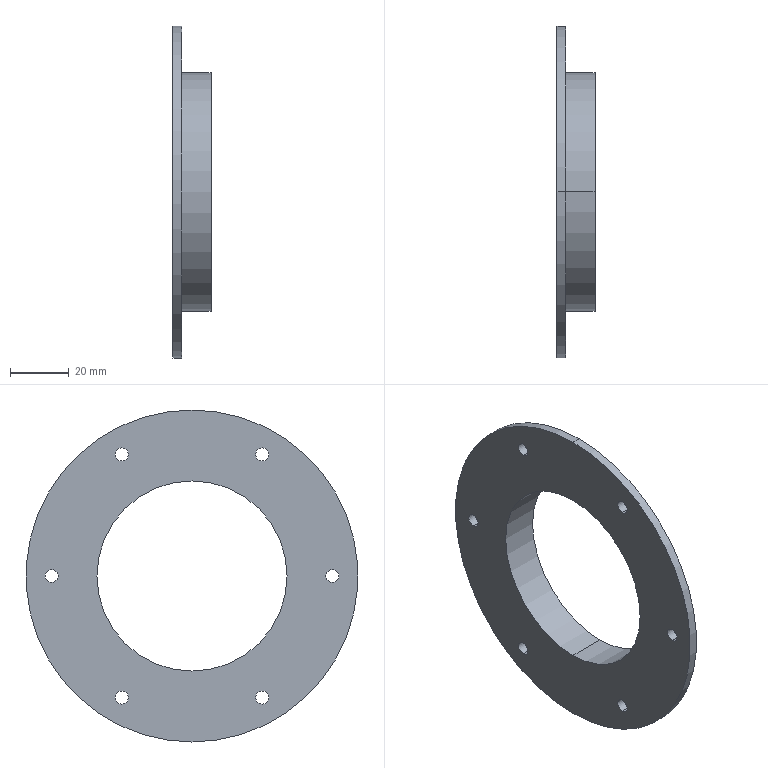Part | SolidWorks | features Chamfer 2, CirPattern 1, ICE 1, Revolution 1 | 1 solid | 31 faces | box 13 x 113.5 x 113.5 mm | volume 34508 mm3 | cylinder 22 | plane 5 | cone 4 | commonest cylinder face diameters 4.5 x12 65 x2 68.6 x2 71.5 x2 81.5 x2 113.5 x2
STEP:
#1=CARTESIAN_POINT('',(0.,24.,43.819));
#2=VERTEX_POINT('',#1);
#3=CARTESIAN_POINT('',(0.,24.,39.319));
#4=VERTEX_POINT('',#3);
#5=CARTESIAN_POINT('',(0.,24.,41.569));
#6=DIRECTION('',(1.,0.,0.));
#7=DIRECTION('',(0.,0.,-1.));
#8=AXIS2_PLACEMENT_3D('',#5,#6,#7);
#9=CIRCLE('',#8,2.25);
#10=EDGE_CURVE('',#2,#4,#9,.T.);
#11=ORIENTED_EDGE('',*,*,#10,.F.);
#12=CARTESIAN_POINT('',(3.,24.,43.819));
#13=VERTEX_POINT('',#12);
#14=CARTESIAN_POINT('',(-7.,24.,43.819));
#15=DIRECTION('',(1.,0.,0.));
#16=VECTOR('',#15,1000.);
#17=LINE('',#14,#16);
#18=EDGE_CURVE('',#2,#13,#17,.T.);
#19=ORIENTED_EDGE('',*,*,#18,.T.);
#20=CARTESIAN_POINT('',(3.,24.,39.319));
#21=VERTEX_POINT('',#20);
#22=CARTESIAN_POINT('',(3.,24.,41.569));
#23=DIRECTION('',(1.,0.,0.));
#24=DIRECTION('',(0.,0.866,-0.5));
#25=AXIS2_PLACEMENT_3D('',#22,#23,#24);
#26=CIRCLE('',#25,2.25);
#27=EDGE_CURVE('',#13,#21,#26,.T.);
#28=ORIENTED_EDGE('',*,*,#27,.T.);
#29=CARTESIAN_POINT('',(-7.,24.,39.319));
#30=DIRECTION('',(1.,0.,0.));
#31=VECTOR('',#30,1000.);
#32=LINE('',#29,#31);
#33=EDGE_CURVE('',#4,#21,#32,.T.);
#34=ORIENTED_EDGE('',*,*,#33,.F.);
#35=EDGE_LOOP('',(#11,#19,#28,#34));
#36=FACE_OUTER_BOUND('',#35,.T.);
#37=CARTESIAN_POINT('',(-7.,24.,41.569));
#38=DIRECTION('',(1.,0.,0.));
#39=DIRECTION('',(0.,0.,-1.));
#40=AXIS2_PLACEMENT_3D('',#37,#38,#39);
#41=CYLINDRICAL_SURFACE('',#40,2.25);
#42=ADVANCED_FACE('',(#36),#41,.F.);
#43=CARTESIAN_POINT('',(0.,-24.,43.819));
#44=VERTEX_POINT('',#43);
#45=CARTESIAN_POINT('',(0.,-24.,39.319));
#46=VERTEX_POINT('',#45);
#47=CARTESIAN_POINT('',(0.,-24.,41.569));
#48=DIRECTION('',(1.,0.,0.));
#49=DIRECTION('',(0.,0.,-1.));
#50=AXIS2_PLACEMENT_3D('',#47,#48,#49);
#51=CIRCLE('',#50,2.25);
#52=EDGE_CURVE('',#44,#46,#51,.T.);
#53=ORIENTED_EDGE('',*,*,#52,.F.);
#54=CARTESIAN_POINT('',(3.,-24.,43.819));
#55=VERTEX_POINT('',#54);
#56=CARTESIAN_POINT('',(-7.,-24.,43.819));
#57=DIRECTION('',(1.,0.,0.));
#58=VECTOR('',#57,1000.);
#59=LINE('',#56,#58);
#60=EDGE_CURVE('',#44,#55,#59,.T.);
#61=ORIENTED_EDGE('',*,*,#60,.T.);
#62=CARTESIAN_POINT('',(3.,-24.,39.319));
#63=VERTEX_POINT('',#62);
#64=CARTESIAN_POINT('',(3.,-24.,41.569));
#65=DIRECTION('',(1.,0.,0.));
#66=DIRECTION('',(0.,0.866,0.5));
#67=AXIS2_PLACEMENT_3D('',#64,#65,#66);
#68=CIRCLE('',#67,2.25);
#69=EDGE_CURVE('',#55,#63,#68,.T.);
#70=ORIENTED_EDGE('',*,*,#69,.T.);
#71=CARTESIAN_POINT('',(-7.,-24.,39.319));
#72=DIRECTION('',(1.,0.,0.));
#73=VECTOR('',#72,1000.);
#74=LINE('',#71,#73);
#75=EDGE_CURVE('',#46,#63,#74,.T.);
#76=ORIENTED_EDGE('',*,*,#75,.F.);
#77=EDGE_LOOP('',(#53,#61,#70,#76));
#78=FACE_OUTER_BOUND('',#77,.T.);
#79=CARTESIAN_POINT('',(-7.,-24.,41.569));
#80=DIRECTION('',(1.,0.,0.));
#81=DIRECTION('',(0.,0.,-1.));
#82=AXIS2_PLACEMENT_3D('',#79,#80,#81);
#83=CYLINDRICAL_SURFACE('',#82,2.25);
#84=ADVANCED_FACE('',(#78),#83,.F.);
#85=CARTESIAN_POINT('',(0.,-48.,2.25));
#86=VERTEX_POINT('',#85);
#87=CARTESIAN_POINT('',(0.,-48.,-2.25));
#88=VERTEX_POINT('',#87);
#89=CARTESIAN_POINT('',(0.,-48.,0.));
#90=DIRECTION('',(1.,0.,0.));
#91=DIRECTION('',(0.,0.,-1.));
#92=AXIS2_PLACEMENT_3D('',#89,#90,#91);
#93=CIRCLE('',#92,2.25);
#94=EDGE_CURVE('',#86,#88,#93,.T.);
#95=ORIENTED_EDGE('',*,*,#94,.F.);
#96=CARTESIAN_POINT('',(3.,-48.,2.25));
#97=VERTEX_POINT('',#96);
#98=CARTESIAN_POINT('',(-7.,-48.,2.25));
#99=DIRECTION('',(1.,0.,0.));
#100=VECTOR('',#99,1000.);
#101=LINE('',#98,#100);
#102=EDGE_CURVE('',#86,#97,#101,.T.);
#103=ORIENTED_EDGE('',*,*,#102,.T.);
#104=CARTESIAN_POINT('',(3.,-48.,-2.25));
#105=VERTEX_POINT('',#104);
#106=CARTESIAN_POINT('',(3.,-48.,0.));
#107=DIRECTION('',(1.,0.,0.));
#108=DIRECTION('',(0.,0.,1.));
#109=AXIS2_PLACEMENT_3D('',#106,#107,#108);
#110=CIRCLE('',#109,2.25);
#111=EDGE_CURVE('',#97,#105,#110,.T.);
#112=ORIENTED_EDGE('',*,*,#111,.T.);
#113=CARTESIAN_POINT('',(-7.,-48.,-2.25));
#114=DIRECTION('',(1.,0.,0.));
#115=VECTOR('',#114,1000.);
#116=LINE('',#113,#115);
#117=EDGE_CURVE('',#88,#105,#116,.T.);
#118=ORIENTED_EDGE('',*,*,#117,.F.);
#119=EDGE_LOOP('',(#95,#103,#112,#118));
#120=FACE_OUTER_BOUND('',#119,.T.);
#121=CARTESIAN_POINT('',(-7.,-48.,0.));
#122=DIRECTION('',(1.,0.,0.));
#123=DIRECTION('',(0.,0.,-1.));
#124=AXIS2_PLACEMENT_3D('',#121,#122,#123);
#125=CYLINDRICAL_SURFACE('',#124,2.25);
#126=ADVANCED_FACE('',(#120),#125,.F.);
#127=CARTESIAN_POINT('',(0.,-24.,-39.319));
#128=VERTEX_POINT('',#127);
#129=CARTESIAN_POINT('',(0.,-24.,-43.819));
#130=VERTEX_POINT('',#129);
#131=CARTESIAN_POINT('',(0.,-24.,-41.569));
#132=DIRECTION('',(1.,0.,0.));
#133=DIRECTION('',(0.,0.,-1.));
#134=AXIS2_PLACEMENT_3D('',#131,#132,#133);
#135=CIRCLE('',#134,2.25);
#136=EDGE_CURVE('',#128,#130,#135,.T.);
#137=ORIENTED_EDGE('',*,*,#136,.F.);
#138=CARTESIAN_POINT('',(3.,-24.,-39.319));
#139=VERTEX_POINT('',#138);
#140=CARTESIAN_POINT('',(-7.,-24.,-39.319));
#141=DIRECTION('',(1.,0.,0.));
#142=VECTOR('',#141,1000.);
#143=LINE('',#140,#142);
#144=EDGE_CURVE('',#128,#139,#143,.T.);
#145=ORIENTED_EDGE('',*,*,#144,.T.);
#146=CARTESIAN_POINT('',(3.,-24.,-43.819));
#147=VERTEX_POINT('',#146);
#148=CARTESIAN_POINT('',(3.,-24.,-41.569));
#149=DIRECTION('',(1.,0.,0.));
#150=DIRECTION('',(0.,-0.866,0.5));
#151=AXIS2_PLACEMENT_3D('',#148,#149,#150);
#152=CIRCLE('',#151,2.25);
#153=EDGE_CURVE('',#139,#147,#152,.T.);
#154=ORIENTED_EDGE('',*,*,#153,.T.);
#155=CARTESIAN_POINT('',(-7.,-24.,-43.819));
#156=DIRECTION('',(1.,0.,0.));
#157=VECTOR('',#156,1000.);
#158=LINE('',#155,#157);
#159=EDGE_CURVE('',#130,#147,#158,.T.);
#160=ORIENTED_EDGE('',*,*,#159,.F.);
#161=EDGE_LOOP('',(#137,#145,#154,#160));
#162=FACE_OUTER_BOUND('',#161,.T.);
#163=CARTESIAN_POINT('',(-7.,-24.,-41.569));
#164=DIRECTION('',(1.,0.,0.));
#165=DIRECTION('',(0.,0.,-1.));
#166=AXIS2_PLACEMENT_3D('',#163,#164,#165);
#167=CYLINDRICAL_SURFACE('',#166,2.25);
#168=ADVANCED_FACE('',(#162),#167,.F.);
#169=CARTESIAN_POINT('',(0.,24.,-39.319));
#170=VERTEX_POINT('',#169);
#171=CARTESIAN_POINT('',(0.,24.,-43.819));
#172=VERTEX_POINT('',#171);
#173=CARTESIAN_POINT('',(0.,24.,-41.569));
#174=DIRECTION('',(1.,0.,0.));
#175=DIRECTION('',(0.,0.,-1.));
#176=AXIS2_PLACEMENT_3D('',#173,#174,#175);
#177=CIRCLE('',#176,2.25);
#178=EDGE_CURVE('',#170,#172,#177,.T.);
#179=ORIENTED_EDGE('',*,*,#178,.F.);
#180=CARTESIAN_POINT('',(3.,24.,-39.319));
#181=VERTEX_POINT('',#180);
#182=CARTESIAN_POINT('',(-7.,24.,-39.319));
#183=DIRECTION('',(1.,0.,0.));
#184=VECTOR('',#183,1000.);
#185=LINE('',#182,#184);
#186=EDGE_CURVE('',#170,#181,#185,.T.);
#187=ORIENTED_EDGE('',*,*,#186,.T.);
#188=CARTESIAN_POINT('',(3.,24.,-43.819));
#189=VERTEX_POINT('',#188);
#190=CARTESIAN_POINT('',(3.,24.,-41.569));
#191=DIRECTION('',(1.,0.,0.));
#192=DIRECTION('',(0.,-0.866,-0.5));
#193=AXIS2_PLACEMENT_3D('',#190,#191,#192);
#194=CIRCLE('',#193,2.25);
#195=EDGE_CURVE('',#181,#189,#194,.T.);
#196=ORIENTED_EDGE('',*,*,#195,.T.);
#197=CARTESIAN_POINT('',(-7.,24.,-43.819));
#198=DIRECTION('',(1.,0.,0.));
#199=VECTOR('',#198,1000.);
#200=LINE('',#197,#199);
#201=EDGE_CURVE('',#172,#189,#200,.T.);
#202=ORIENTED_EDGE('',*,*,#201,.F.);
#203=EDGE_LOOP('',(#179,#187,#196,#202));
#204=FACE_OUTER_BOUND('',#203,.T.);
#205=CARTESIAN_POINT('',(-7.,24.,-41.569));
#206=DIRECTION('',(1.,0.,0.));
#207=DIRECTION('',(0.,0.,-1.));
#208=AXIS2_PLACEMENT_3D('',#205,#206,#207);
#209=CYLINDRICAL_SURFACE('',#208,2.25);
#210=ADVANCED_FACE('',(#204),#209,.F.);
#211=CARTESIAN_POINT('',(0.,48.,2.25));
#212=VERTEX_POINT('',#211);
#213=CARTESIAN_POINT('',(0.,48.,-2.25));
#214=VERTEX_POINT('',#213);
#215=CARTESIAN_POINT('',(0.,48.,0.));
#216=DIRECTION('',(1.,0.,0.));
#217=DIRECTION('',(0.,0.,-1.));
#218=AXIS2_PLACEMENT_3D('',#215,#216,#217);
#219=CIRCLE('',#218,2.25);
#220=EDGE_CURVE('',#212,#214,#219,.T.);
#221=ORIENTED_EDGE('',*,*,#220,.F.);
#222=CARTESIAN_POINT('',(3.,48.,2.25));
#223=VERTEX_POINT('',#222);
#224=CARTESIAN_POINT('',(-7.,48.,2.25));
#225=DIRECTION('',(1.,0.,0.));
#226=VECTOR('',#225,1000.);
#227=LINE('',#224,#226);
#228=EDGE_CURVE('',#212,#223,#227,.T.);
#229=ORIENTED_EDGE('',*,*,#228,.T.);
#230=CARTESIAN_POINT('',(3.,48.,-2.25));
#231=VERTEX_POINT('',#230);
#232=CARTESIAN_POINT('',(3.,48.,0.));
#233=DIRECTION('',(1.,0.,0.));
#234=DIRECTION('',(0.,0.,-1.));
#235=AXIS2_PLACEMENT_3D('',#232,#233,#234);
#236=CIRCLE('',#235,2.25);
#237=EDGE_CURVE('',#223,#231,#236,.T.);
#238=ORIENTED_EDGE('',*,*,#237,.T.);
#239=CARTESIAN_POINT('',(-7.,48.,-2.25));
#240=DIRECTION('',(1.,0.,0.));
#241=VECTOR('',#240,1000.);
#242=LINE('',#239,#241);
#243=EDGE_CURVE('',#214,#231,#242,.T.);
#244=ORIENTED_EDGE('',*,*,#243,.F.);
#245=EDGE_LOOP('',(#221,#229,#238,#244));
#246=FACE_OUTER_BOUND('',#245,.T.);
#247=CARTESIAN_POINT('',(-7.,48.,0.));
#248=DIRECTION('',(1.,0.,0.));
#249=DIRECTION('',(0.,0.,-1.));
#250=AXIS2_PLACEMENT_3D('',#247,#248,#249);
#251=CYLINDRICAL_SURFACE('',#250,2.25);
#252=ADVANCED_FACE('',(#246),#251,.F.);
#253=CARTESIAN_POINT('',(13.,0.,-33.3));
#254=VERTEX_POINT('',#253);
#255=CARTESIAN_POINT('',(13.,0.,33.3));
#256=VERTEX_POINT('',#255);
#257=CARTESIAN_POINT('',(13.,0.,0.));
#258=DIRECTION('',(1.,0.,0.));
#259=DIRECTION('',(0.,0.,1.));
#260=AXIS2_PLACEMENT_3D('',#257,#258,#259);
#261=CIRCLE('',#260,33.3);
#262=EDGE_CURVE('',#254,#256,#261,.T.);
#263=ORIENTED_EDGE('',*,*,#262,.F.);
#264=CARTESIAN_POINT('',(12.,0.,-34.3));
#265=VERTEX_POINT('',#264);
#266=CARTESIAN_POINT('',(12.,0.,-34.3));
#267=DIRECTION('',(-0.7071,0.,-0.7071));
#268=VECTOR('',#267,1000.);
#269=LINE('',#266,#268);
#270=EDGE_CURVE('',#254,#265,#269,.T.);
#271=ORIENTED_EDGE('',*,*,#270,.T.);
#272=CARTESIAN_POINT('',(12.,0.,34.3));
#273=VERTEX_POINT('',#272);
#274=CARTESIAN_POINT('',(12.,0.,0.));
#275=DIRECTION('',(-1.,0.,0.));
#276=DIRECTION('',(0.,0.,1.));
#277=AXIS2_PLACEMENT_3D('',#274,#275,#276);
#278=CIRCLE('',#277,34.3);
#279=EDGE_CURVE('',#273,#265,#278,.T.);
#280=ORIENTED_EDGE('',*,*,#279,.F.);
#281=CARTESIAN_POINT('',(12.,0.,34.3));
#282=DIRECTION('',(-0.7071,0.,0.7071));
#283=VECTOR('',#282,1000.);
#284=LINE('',#281,#283);
#285=EDGE_CURVE('',#256,#273,#284,.T.);
#286=ORIENTED_EDGE('',*,*,#285,.F.);
#287=EDGE_LOOP('',(#263,#271,#280,#286));
#288=FACE_OUTER_BOUND('',#287,.T.);
#289=CARTESIAN_POINT('',(12.,0.,0.));
#290=DIRECTION('',(-1.,0.,0.));
#291=DIRECTION('',(0.,0.,1.));
#292=AXIS2_PLACEMENT_3D('',#289,#290,#291);
#293=CONICAL_SURFACE('',#292,34.3,0.7854);
#294=ADVANCED_FACE('',(#288),#293,.T.);
#295=CARTESIAN_POINT('',(9.,0.,35.75));
#296=VERTEX_POINT('',#295);
#297=CARTESIAN_POINT('',(9.,0.,-35.75));
#298=VERTEX_POINT('',#297);
#299=CARTESIAN_POINT('',(9.,0.,0.));
#300=DIRECTION('',(1.,0.,0.));
#301=DIRECTION('',(0.,0.,1.));
#302=AXIS2_PLACEMENT_3D('',#299,#300,#301);
#303=CIRCLE('',#302,35.75);
#304=EDGE_CURVE('',#296,#298,#303,.T.);
#305=ORIENTED_EDGE('',*,*,#304,.F.);
#306=CARTESIAN_POINT('',(13.,0.,38.551));
#307=VERTEX_POINT('',#306);
#308=CARTESIAN_POINT('',(13.,0.,38.551));
#309=DIRECTION('',(0.8192,0.,0.5736));
#310=VECTOR('',#309,1000.);
#311=LINE('',#308,#310);
#312=EDGE_CURVE('',#296,#307,#311,.T.);
#313=ORIENTED_EDGE('',*,*,#312,.T.);
#314=CARTESIAN_POINT('',(13.,0.,-38.551));
#315=VERTEX_POINT('',#314);
#316=CARTESIAN_POINT('',(13.,0.,0.));
#317=DIRECTION('',(-1.,0.,0.));
#318=DIRECTION('',(0.,0.,1.));
#319=AXIS2_PLACEMENT_3D('',#316,#317,#318);
#320=CIRCLE('',#319,38.551);
#321=EDGE_CURVE('',#315,#307,#320,.T.);
#322=ORIENTED_EDGE('',*,*,#321,.F.);
#323=CARTESIAN_POINT('',(13.,0.,-38.551));
#324=DIRECTION('',(0.8192,0.,-0.5736));
#325=VECTOR('',#324,1000.);
#326=LINE('',#323,#325);
#327=EDGE_CURVE('',#298,#315,#326,.T.);
#328=ORIENTED_EDGE('',*,*,#327,.F.);
#329=EDGE_LOOP('',(#305,#313,#322,#328));
#330=FACE_OUTER_BOUND('',#329,.T.);
#331=CARTESIAN_POINT('',(13.,0.,0.));
#332=DIRECTION('',(1.,0.,0.));
#333=DIRECTION('',(0.,0.,-1.));
#334=AXIS2_PLACEMENT_3D('',#331,#332,#333);
#335=CONICAL_SURFACE('',#334,38.551,0.6109);
#336=ADVANCED_FACE('',(#330),#335,.F.);
#337=CARTESIAN_POINT('',(3.,0.,56.75));
#338=VERTEX_POINT('',#337);
#339=CARTESIAN_POINT('',(3.,0.,-56.75));
#340=VERTEX_POINT('',#339);
#341=CARTESIAN_POINT('',(3.,0.,0.));
#342=DIRECTION('',(-1.,0.,0.));
#343=DIRECTION('',(0.,0.,1.));
#344=AXIS2_PLACEMENT_3D('',#341,#342,#343);
#345=CIRCLE('',#344,56.75);
#346=EDGE_CURVE('',#338,#340,#345,.T.);
#347=ORIENTED_EDGE('',*,*,#346,.T.);
#348=CARTESIAN_POINT('',(0.,0.,-56.75));
#349=VERTEX_POINT('',#348);
#350=CARTESIAN_POINT('',(0.,0.,-56.75));
#351=DIRECTION('',(-1.,0.,0.));
#352=VECTOR('',#351,1000.);
#353=LINE('',#350,#352);
#354=EDGE_CURVE('',#340,#349,#353,.T.);
#355=ORIENTED_EDGE('',*,*,#354,.T.);
#356=CARTESIAN_POINT('',(0.,0.,56.75));
#357=VERTEX_POINT('',#356);
#358=CARTESIAN_POINT('',(0.,0.,0.));
#359=DIRECTION('',(-1.,0.,0.));
#360=DIRECTION('',(0.,0.,1.));
#361=AXIS2_PLACEMENT_3D('',#358,#359,#360);
#362=CIRCLE('',#361,56.75);
#363=EDGE_CURVE('',#357,#349,#362,.T.);
#364=ORIENTED_EDGE('',*,*,#363,.F.);
#365=CARTESIAN_POINT('',(0.,0.,56.75));
#366=DIRECTION('',(-1.,0.,0.));
#367=VECTOR('',#366,1000.);
#368=LINE('',#365,#367);
#369=EDGE_CURVE('',#338,#357,#368,.T.);
#370=ORIENTED_EDGE('',*,*,#369,.F.);
#371=EDGE_LOOP('',(#347,#355,#364,#370));
#372=FACE_OUTER_BOUND('',#371,.T.);
#373=CARTESIAN_POINT('',(0.,0.,0.));
#374=DIRECTION('',(-1.,0.,0.));
#375=DIRECTION('',(0.,0.,1.));
#376=AXIS2_PLACEMENT_3D('',#373,#374,#375);
#377=CYLINDRICAL_SURFACE('',#376,56.75);
#378=ADVANCED_FACE('',(#372),#377,.T.);
#379=CARTESIAN_POINT('',(13.,0.,40.75));
#380=VERTEX_POINT('',#379);
#381=CARTESIAN_POINT('',(13.,0.,-40.75));
#382=VERTEX_POINT('',#381);
#383=CARTESIAN_POINT('',(13.,0.,0.));
#384=DIRECTION('',(-1.,0.,0.));
#385=DIRECTION('',(0.,0.,1.));
#386=AXIS2_PLACEMENT_3D('',#383,#384,#385);
#387=CIRCLE('',#386,40.75);
#388=EDGE_CURVE('',#380,#382,#387,.T.);
#389=ORIENTED_EDGE('',*,*,#388,.T.);
#390=CARTESIAN_POINT('',(3.,0.,-40.75));
#391=VERTEX_POINT('',#390);
#392=CARTESIAN_POINT('',(0.,0.,-40.75));
#393=DIRECTION('',(-1.,0.,0.));
#394=VECTOR('',#393,1000.);
#395=LINE('',#392,#394);
#396=EDGE_CURVE('',#382,#391,#395,.T.);
#397=ORIENTED_EDGE('',*,*,#396,.T.);
#398=CARTESIAN_POINT('',(3.,0.,40.75));
#399=VERTEX_POINT('',#398);
#400=CARTESIAN_POINT('',(3.,0.,0.));
#401=DIRECTION('',(-1.,0.,0.));
#402=DIRECTION('',(0.,0.,1.));
#403=AXIS2_PLACEMENT_3D('',#400,#401,#402);
#404=CIRCLE('',#403,40.75);
#405=EDGE_CURVE('',#399,#391,#404,.T.);
#406=ORIENTED_EDGE('',*,*,#405,.F.);
#407=CARTESIAN_POINT('',(0.,0.,40.75));
#408=DIRECTION('',(-1.,0.,0.));
#409=VECTOR('',#408,1000.);
#410=LINE('',#407,#409);
#411=EDGE_CURVE('',#380,#399,#410,.T.);
#412=ORIENTED_EDGE('',*,*,#411,.F.);
#413=EDGE_LOOP('',(#389,#397,#406,#412));
#414=FACE_OUTER_BOUND('',#413,.T.);
#415=CARTESIAN_POINT('',(0.,0.,0.));
#416=DIRECTION('',(-1.,0.,0.));
#417=DIRECTION('',(0.,0.,1.));
#418=AXIS2_PLACEMENT_3D('',#415,#416,#417);
#419=CYLINDRICAL_SURFACE('',#418,40.75);
#420=ADVANCED_FACE('',(#414),#419,.T.);
#421=ORIENTED_EDGE('',*,*,#304,.T.);
#422=CARTESIAN_POINT('',(3.,0.,-35.75));
#423=VERTEX_POINT('',#422);
#424=CARTESIAN_POINT('',(0.,0.,-35.75));
#425=DIRECTION('',(-1.,0.,0.));
#426=VECTOR('',#425,1000.);
#427=LINE('',#424,#426);
#428=EDGE_CURVE('',#298,#423,#427,.T.);
#429=ORIENTED_EDGE('',*,*,#428,.T.);
#430=CARTESIAN_POINT('',(3.,0.,35.75));
#431=VERTEX_POINT('',#430);
#432=CARTESIAN_POINT('',(3.,0.,0.));
#433=DIRECTION('',(-1.,0.,0.));
#434=DIRECTION('',(0.,0.,1.));
#435=AXIS2_PLACEMENT_3D('',#432,#433,#434);
#436=CIRCLE('',#435,35.75);
#437=EDGE_CURVE('',#423,#431,#436,.T.);
#438=ORIENTED_EDGE('',*,*,#437,.T.);
#439=CARTESIAN_POINT('',(0.,0.,35.75));
#440=DIRECTION('',(-1.,0.,0.));
#441=VECTOR('',#440,1000.);
#442=LINE('',#439,#441);
#443=EDGE_CURVE('',#296,#431,#442,.T.);
#444=ORIENTED_EDGE('',*,*,#443,.F.);
#445=EDGE_LOOP('',(#421,#429,#438,#444));
#446=FACE_OUTER_BOUND('',#445,.T.);
#447=CARTESIAN_POINT('',(0.,0.,0.));
#448=DIRECTION('',(-1.,0.,0.));
#449=DIRECTION('',(0.,0.,1.));
#450=AXIS2_PLACEMENT_3D('',#447,#448,#449);
#451=CYLINDRICAL_SURFACE('',#450,35.75);
#452=ADVANCED_FACE('',(#446),#451,.F.);
#453=ORIENTED_EDGE('',*,*,#279,.T.);
#454=CARTESIAN_POINT('',(3.,0.,-34.3));
#455=VERTEX_POINT('',#454);
#456=CARTESIAN_POINT('',(0.,0.,-34.3));
#457=DIRECTION('',(-1.,0.,0.));
#458=VECTOR('',#457,1000.);
#459=LINE('',#456,#458);
#460=EDGE_CURVE('',#265,#455,#459,.T.);
#461=ORIENTED_EDGE('',*,*,#460,.T.);
#462=CARTESIAN_POINT('',(3.,0.,34.3));
#463=VERTEX_POINT('',#462);
#464=CARTESIAN_POINT('',(3.,0.,0.));
#465=DIRECTION('',(-1.,0.,0.));
#466=DIRECTION('',(0.,0.,1.));
#467=AXIS2_PLACEMENT_3D('',#464,#465,#466);
#468=CIRCLE('',#467,34.3);
#469=EDGE_CURVE('',#463,#455,#468,.T.);
#470=ORIENTED_EDGE('',*,*,#469,.F.);
#471=CARTESIAN_POINT('',(0.,0.,34.3));
#472=DIRECTION('',(-1.,0.,0.));
#473=VECTOR('',#472,1000.);
#474=LINE('',#471,#473);
#475=EDGE_CURVE('',#273,#463,#474,.T.);
#476=ORIENTED_EDGE('',*,*,#475,.F.);
#477=EDGE_LOOP('',(#453,#461,#470,#476));
#478=FACE_OUTER_BOUND('',#477,.T.);
#479=CARTESIAN_POINT('',(0.,0.,0.));
#480=DIRECTION('',(-1.,0.,0.));
#481=DIRECTION('',(0.,0.,1.));
#482=AXIS2_PLACEMENT_3D('',#479,#480,#481);
#483=CYLINDRICAL_SURFACE('',#482,34.3);
#484=ADVANCED_FACE('',(#478),#483,.T.);
#485=CARTESIAN_POINT('',(13.,0.,-32.5));
#486=VERTEX_POINT('',#485);
#487=CARTESIAN_POINT('',(13.,0.,32.5));
#488=VERTEX_POINT('',#487);
#489=CARTESIAN_POINT('',(13.,0.,0.));
#490=DIRECTION('',(-1.,0.,0.));
#491=DIRECTION('',(0.,0.,1.));
#492=AXIS2_PLACEMENT_3D('',#489,#490,#491);
#493=CIRCLE('',#492,32.5);
#494=EDGE_CURVE('',#486,#488,#493,.T.);
#495=ORIENTED_EDGE('',*,*,#494,.F.);
#496=CARTESIAN_POINT('',(0.,0.,-32.5));
#497=VERTEX_POINT('',#496);
#498=CARTESIAN_POINT('',(0.,0.,-32.5));
#499=DIRECTION('',(-1.,0.,0.));
#500=VECTOR('',#499,1000.);
#501=LINE('',#498,#500);
#502=EDGE_CURVE('',#486,#497,#501,.T.);
#503=ORIENTED_EDGE('',*,*,#502,.T.);
#504=CARTESIAN_POINT('',(0.,0.,32.5));
#505=VERTEX_POINT('',#504);
#506=CARTESIAN_POINT('',(0.,0.,0.));
#507=DIRECTION('',(-1.,0.,0.));
#508=DIRECTION('',(0.,0.,1.));
#509=AXIS2_PLACEMENT_3D('',#506,#507,#508);
#510=CIRCLE('',#509,32.5);
#511=EDGE_CURVE('',#497,#505,#510,.T.);
#512=ORIENTED_EDGE('',*,*,#511,.T.);
#513=CARTESIAN_POINT('',(0.,0.,32.5));
#514=DIRECTION('',(-1.,0.,0.));
#515=VECTOR('',#514,1000.);
#516=LINE('',#513,#515);
#517=EDGE_CURVE('',#488,#505,#516,.T.);
#518=ORIENTED_EDGE('',*,*,#517,.F.);
#519=EDGE_LOOP('',(#495,#503,#512,#518));
#520=FACE_OUTER_BOUND('',#519,.T.);
#521=CARTESIAN_POINT('',(0.,0.,0.));
#522=DIRECTION('',(-1.,0.,0.));
#523=DIRECTION('',(0.,0.,1.));
#524=AXIS2_PLACEMENT_3D('',#521,#522,#523);
#525=CYLINDRICAL_SURFACE('',#524,32.5);
#526=ADVANCED_FACE('',(#520),#525,.F.);
#527=CARTESIAN_POINT('',(0.,24.,41.569));
#528=DIRECTION('',(1.,0.,0.));
#529=DIRECTION('',(0.,0.,-1.));
#530=AXIS2_PLACEMENT_3D('',#527,#528,#529);
#531=CIRCLE('',#530,2.25);
#532=EDGE_CURVE('',#4,#2,#531,.T.);
#533=ORIENTED_EDGE('',*,*,#532,.T.);
#534=ORIENTED_EDGE('',*,*,#10,.T.);
#535=EDGE_LOOP('',(#533,#534));
#536=FACE_BOUND('',#535,.T.);
#537=CARTESIAN_POINT('',(0.,-24.,41.569));
#538=DIRECTION('',(1.,0.,0.));
#539=DIRECTION('',(0.,0.,-1.));
#540=AXIS2_PLACEMENT_3D('',#537,#538,#539);
#541=CIRCLE('',#540,2.25);
#542=EDGE_CURVE('',#46,#44,#541,.T.);
#543=ORIENTED_EDGE('',*,*,#542,.T.);
#544=ORIENTED_EDGE('',*,*,#52,.T.);
#545=EDGE_LOOP('',(#543,#544));
#546=FACE_BOUND('',#545,.T.);
#547=CARTESIAN_POINT('',(0.,-48.,0.));
#548=DIRECTION('',(1.,0.,0.));
#549=DIRECTION('',(0.,0.,-1.));
#550=AXIS2_PLACEMENT_3D('',#547,#548,#549);
#551=CIRCLE('',#550,2.25);
#552=EDGE_CURVE('',#88,#86,#551,.T.);
#553=ORIENTED_EDGE('',*,*,#552,.T.);
#554=ORIENTED_EDGE('',*,*,#94,.T.);
#555=EDGE_LOOP('',(#553,#554));
#556=FACE_BOUND('',#555,.T.);
#557=CARTESIAN_POINT('',(0.,-24.,-41.569));
#558=DIRECTION('',(1.,0.,0.));
#559=DIRECTION('',(0.,0.,-1.));
#560=AXIS2_PLACEMENT_3D('',#557,#558,#559);
#561=CIRCLE('',#560,2.25);
#562=EDGE_CURVE('',#130,#128,#561,.T.);
#563=ORIENTED_EDGE('',*,*,#562,.T.);
#564=ORIENTED_EDGE('',*,*,#136,.T.);
#565=EDGE_LOOP('',(#563,#564));
#566=FACE_BOUND('',#565,.T.);
#567=CARTESIAN_POINT('',(0.,24.,-41.569));
#568=DIRECTION('',(1.,0.,0.));
#569=DIRECTION('',(0.,0.,-1.));
#570=AXIS2_PLACEMENT_3D('',#567,#568,#569);
#571=CIRCLE('',#570,2.25);
#572=EDGE_CURVE('',#172,#170,#571,.T.);
#573=ORIENTED_EDGE('',*,*,#572,.T.);
#574=ORIENTED_EDGE('',*,*,#178,.T.);
#575=EDGE_LOOP('',(#573,#574));
#576=FACE_BOUND('',#575,.T.);
#577=CARTESIAN_POINT('',(0.,48.,0.));
#578=DIRECTION('',(1.,0.,0.));
#579=DIRECTION('',(0.,0.,-1.));
#580=AXIS2_PLACEMENT_3D('',#577,#578,#579);
#581=CIRCLE('',#580,2.25);
#582=EDGE_CURVE('',#214,#212,#581,.T.);
#583=ORIENTED_EDGE('',*,*,#582,.T.);
#584=ORIENTED_EDGE('',*,*,#220,.T.);
#585=EDGE_LOOP('',(#583,#584));
#586=FACE_BOUND('',#585,.T.);
#587=CARTESIAN_POINT('',(0.,0.,0.));
#588=DIRECTION('',(-1.,0.,0.));
#589=DIRECTION('',(0.,0.,1.));
#590=AXIS2_PLACEMENT_3D('',#587,#588,#589);
#591=CIRCLE('',#590,32.5);
#592=EDGE_CURVE('',#505,#497,#591,.T.);
#593=ORIENTED_EDGE('',*,*,#592,.F.);
#594=ORIENTED_EDGE('',*,*,#511,.F.);
#595=EDGE_LOOP('',(#593,#594));
#596=FACE_BOUND('',#595,.T.);
#597=ORIENTED_EDGE('',*,*,#363,.T.);
#598=CARTESIAN_POINT('',(0.,0.,0.));
#599=DIRECTION('',(-1.,0.,0.));
#600=DIRECTION('',(0.,0.,1.));
#601=AXIS2_PLACEMENT_3D('',#598,#599,#600);
#602=CIRCLE('',#601,56.75);
#603=EDGE_CURVE('',#349,#357,#602,.T.);
#604=ORIENTED_EDGE('',*,*,#603,.T.);
#605=EDGE_LOOP('',(#597,#604));
#606=FACE_OUTER_BOUND('',#605,.T.);
#607=CARTESIAN_POINT('',(0.,56.75,0.));
#608=DIRECTION('',(1.,0.,0.));
#609=DIRECTION('',(0.,0.,-1.));
#610=AXIS2_PLACEMENT_3D('',#607,#608,#609);
#611=PLANE('',#610);
#612=ADVANCED_FACE('',(#536,#546,#556,#566,#576,#586,#596,#606),#611,.F.);
#613=ORIENTED_EDGE('',*,*,#502,.F.);
#614=CARTESIAN_POINT('',(13.,0.,0.));
#615=DIRECTION('',(-1.,0.,0.));
#616=DIRECTION('',(0.,0.,1.));
#617=AXIS2_PLACEMENT_3D('',#614,#615,#616);
#618=CIRCLE('',#617,32.5);
#619=EDGE_CURVE('',#488,#486,#618,.T.);
#620=ORIENTED_EDGE('',*,*,#619,.F.);
#621=ORIENTED_EDGE('',*,*,#517,.T.);
#622=ORIENTED_EDGE('',*,*,#592,.T.);
#623=EDGE_LOOP('',(#613,#620,#621,#622));
#624=FACE_OUTER_BOUND('',#623,.T.);
#625=CARTESIAN_POINT('',(0.,0.,0.));
#626=DIRECTION('',(-1.,0.,0.));
#627=DIRECTION('',(0.,0.,1.));
#628=AXIS2_PLACEMENT_3D('',#625,#626,#627);
#629=CYLINDRICAL_SURFACE('',#628,32.5);
#630=ADVANCED_FACE('',(#624),#629,.F.);
#631=CARTESIAN_POINT('',(13.,0.,0.));
#632=DIRECTION('',(1.,0.,0.));
#633=DIRECTION('',(0.,0.,1.));
#634=AXIS2_PLACEMENT_3D('',#631,#632,#633);
#635=CIRCLE('',#634,33.3);
#636=EDGE_CURVE('',#256,#254,#635,.T.);
#637=ORIENTED_EDGE('',*,*,#636,.T.);
#638=ORIENTED_EDGE('',*,*,#262,.T.);
#639=EDGE_LOOP('',(#637,#638));
#640=FACE_OUTER_BOUND('',#639,.T.);
#641=ORIENTED_EDGE('',*,*,#619,.T.);
#642=ORIENTED_EDGE('',*,*,#494,.T.);
#643=EDGE_LOOP('',(#641,#642));
#644=FACE_BOUND('',#643,.T.);
#645=CARTESIAN_POINT('',(13.,32.5,0.));
#646=DIRECTION('',(-1.,0.,0.));
#647=DIRECTION('',(0.,0.,1.));
#648=AXIS2_PLACEMENT_3D('',#645,#646,#647);
#649=PLANE('',#648);
#650=ADVANCED_FACE('',(#640,#644),#649,.F.);
#651=ORIENTED_EDGE('',*,*,#460,.F.);
#652=CARTESIAN_POINT('',(12.,0.,0.));
#653=DIRECTION('',(-1.,0.,0.));
#654=DIRECTION('',(0.,0.,1.));
#655=AXIS2_PLACEMENT_3D('',#652,#653,#654);
#656=CIRCLE('',#655,34.3);
#657=EDGE_CURVE('',#265,#273,#656,.T.);
#658=ORIENTED_EDGE('',*,*,#657,.T.);
#659=ORIENTED_EDGE('',*,*,#475,.T.);
#660=CARTESIAN_POINT('',(3.,0.,0.));
#661=DIRECTION('',(-1.,0.,0.));
#662=DIRECTION('',(0.,0.,1.));
#663=AXIS2_PLACEMENT_3D('',#660,#661,#662);
#664=CIRCLE('',#663,34.3);
#665=EDGE_CURVE('',#455,#463,#664,.T.);
#666=ORIENTED_EDGE('',*,*,#665,.F.);
#667=EDGE_LOOP('',(#651,#658,#659,#666));
#668=FACE_OUTER_BOUND('',#667,.T.);
#669=CARTESIAN_POINT('',(0.,0.,0.));
#670=DIRECTION('',(-1.,0.,0.));
#671=DIRECTION('',(0.,0.,1.));
#672=AXIS2_PLACEMENT_3D('',#669,#670,#671);
#673=CYLINDRICAL_SURFACE('',#672,34.3);
#674=ADVANCED_FACE('',(#668),#673,.T.);
#675=CARTESIAN_POINT('',(3.,0.,0.));
#676=DIRECTION('',(-1.,0.,0.));
#677=DIRECTION('',(0.,0.,1.));
#678=AXIS2_PLACEMENT_3D('',#675,#676,#677);
#679=CIRCLE('',#678,35.75);
#680=EDGE_CURVE('',#431,#423,#679,.T.);
#681=ORIENTED_EDGE('',*,*,#680,.F.);
#682=ORIENTED_EDGE('',*,*,#437,.F.);
#683=EDGE_LOOP('',(#681,#682));
#684=FACE_OUTER_BOUND('',#683,.T.);
#685=ORIENTED_EDGE('',*,*,#469,.T.);
#686=ORIENTED_EDGE('',*,*,#665,.T.);
#687=EDGE_LOOP('',(#685,#686));
#688=FACE_BOUND('',#687,.T.);
#689=CARTESIAN_POINT('',(3.,34.3,0.));
#690=DIRECTION('',(-1.,0.,0.));
#691=DIRECTION('',(0.,0.,1.));
#692=AXIS2_PLACEMENT_3D('',#689,#690,#691);
#693=PLANE('',#692);
#694=ADVANCED_FACE('',(#684,#688),#693,.F.);
#695=ORIENTED_EDGE('',*,*,#428,.F.);
#696=CARTESIAN_POINT('',(9.,0.,0.));
#697=DIRECTION('',(1.,0.,0.));
#698=DIRECTION('',(0.,0.,1.));
#699=AXIS2_PLACEMENT_3D('',#696,#697,#698);
#700=CIRCLE('',#699,35.75);
#701=EDGE_CURVE('',#298,#296,#700,.T.);
#702=ORIENTED_EDGE('',*,*,#701,.T.);
#703=ORIENTED_EDGE('',*,*,#443,.T.);
#704=ORIENTED_EDGE('',*,*,#680,.T.);
#705=EDGE_LOOP('',(#695,#702,#703,#704));
#706=FACE_OUTER_BOUND('',#705,.T.);
#707=CARTESIAN_POINT('',(0.,0.,0.));
#708=DIRECTION('',(-1.,0.,0.));
#709=DIRECTION('',(0.,0.,1.));
#710=AXIS2_PLACEMENT_3D('',#707,#708,#709);
#711=CYLINDRICAL_SURFACE('',#710,35.75);
#712=ADVANCED_FACE('',(#706),#711,.F.);
#713=ORIENTED_EDGE('',*,*,#321,.T.);
#714=CARTESIAN_POINT('',(13.,0.,0.));
#715=DIRECTION('',(-1.,0.,0.));
#716=DIRECTION('',(0.,0.,1.));
#717=AXIS2_PLACEMENT_3D('',#714,#715,#716);
#718=CIRCLE('',#717,38.551);
#719=EDGE_CURVE('',#307,#315,#718,.T.);
#720=ORIENTED_EDGE('',*,*,#719,.T.);
#721=EDGE_LOOP('',(#713,#720));
#722=FACE_BOUND('',#721,.T.);
#723=ORIENTED_EDGE('',*,*,#388,.F.);
#724=CARTESIAN_POINT('',(13.,0.,0.));
#725=DIRECTION('',(-1.,0.,0.));
#726=DIRECTION('',(0.,0.,1.));
#727=AXIS2_PLACEMENT_3D('',#724,#725,#726);
#728=CIRCLE('',#727,40.75);
#729=EDGE_CURVE('',#382,#380,#728,.T.);
#730=ORIENTED_EDGE('',*,*,#729,.F.);
#731=EDGE_LOOP('',(#723,#730));
#732=FACE_OUTER_BOUND('',#731,.T.);
#733=CARTESIAN_POINT('',(13.,35.75,0.));
#734=DIRECTION('',(-1.,0.,0.));
#735=DIRECTION('',(0.,0.,1.));
#736=AXIS2_PLACEMENT_3D('',#733,#734,#735);
#737=PLANE('',#736);
#738=ADVANCED_FACE('',(#722,#732),#737,.F.);
#739=ORIENTED_EDGE('',*,*,#396,.F.);
#740=ORIENTED_EDGE('',*,*,#729,.T.);
#741=ORIENTED_EDGE('',*,*,#411,.T.);
#742=CARTESIAN_POINT('',(3.,0.,0.));
#743=DIRECTION('',(-1.,0.,0.));
#744=DIRECTION('',(0.,0.,1.));
#745=AXIS2_PLACEMENT_3D('',#742,#743,#744);
#746=CIRCLE('',#745,40.75);
#747=EDGE_CURVE('',#391,#399,#746,.T.);
#748=ORIENTED_EDGE('',*,*,#747,.F.);
#749=EDGE_LOOP('',(#739,#740,#741,#748));
#750=FACE_OUTER_BOUND('',#749,.T.);
#751=CARTESIAN_POINT('',(0.,0.,0.));
#752=DIRECTION('',(-1.,0.,0.));
#753=DIRECTION('',(0.,0.,1.));
#754=AXIS2_PLACEMENT_3D('',#751,#752,#753);
#755=CYLINDRICAL_SURFACE('',#754,40.75);
#756=ADVANCED_FACE('',(#750),#755,.T.);
#757=CARTESIAN_POINT('',(3.,24.,41.569));
#758=DIRECTION('',(1.,0.,0.));
#759=DIRECTION('',(0.,0.866,-0.5));
#760=AXIS2_PLACEMENT_3D('',#757,#758,#759);
#761=CIRCLE('',#760,2.25);
#762=EDGE_CURVE('',#21,#13,#761,.T.);
#763=ORIENTED_EDGE('',*,*,#762,.F.);
#764=ORIENTED_EDGE('',*,*,#27,.F.);
#765=EDGE_LOOP('',(#763,#764));
#766=FACE_BOUND('',#765,.T.);
#767=CARTESIAN_POINT('',(3.,-24.,41.569));
#768=DIRECTION('',(1.,0.,0.));
#769=DIRECTION('',(0.,0.866,0.5));
#770=AXIS2_PLACEMENT_3D('',#767,#768,#769);
#771=CIRCLE('',#770,2.25);
#772=EDGE_CURVE('',#63,#55,#771,.T.);
#773=ORIENTED_EDGE('',*,*,#772,.F.);
#774=ORIENTED_EDGE('',*,*,#69,.F.);
#775=EDGE_LOOP('',(#773,#774));
#776=FACE_BOUND('',#775,.T.);
#777=CARTESIAN_POINT('',(3.,-48.,0.));
#778=DIRECTION('',(1.,0.,0.));
#779=DIRECTION('',(0.,0.,1.));
#780=AXIS2_PLACEMENT_3D('',#777,#778,#779);
#781=CIRCLE('',#780,2.25);
#782=EDGE_CURVE('',#105,#97,#781,.T.);
#783=ORIENTED_EDGE('',*,*,#782,.F.);
#784=ORIENTED_EDGE('',*,*,#111,.F.);
#785=EDGE_LOOP('',(#783,#784));
#786=FACE_BOUND('',#785,.T.);
#787=CARTESIAN_POINT('',(3.,-24.,-41.569));
#788=DIRECTION('',(1.,0.,0.));
#789=DIRECTION('',(0.,-0.866,0.5));
#790=AXIS2_PLACEMENT_3D('',#787,#788,#789);
#791=CIRCLE('',#790,2.25);
#792=EDGE_CURVE('',#147,#139,#791,.T.);
#793=ORIENTED_EDGE('',*,*,#792,.F.);
#794=ORIENTED_EDGE('',*,*,#153,.F.);
#795=EDGE_LOOP('',(#793,#794));
#796=FACE_BOUND('',#795,.T.);
#797=CARTESIAN_POINT('',(3.,24.,-41.569));
#798=DIRECTION('',(1.,0.,0.));
#799=DIRECTION('',(0.,-0.866,-0.5));
#800=AXIS2_PLACEMENT_3D('',#797,#798,#799);
#801=CIRCLE('',#800,2.25);
#802=EDGE_CURVE('',#189,#181,#801,.T.);
#803=ORIENTED_EDGE('',*,*,#802,.F.);
#804=ORIENTED_EDGE('',*,*,#195,.F.);
#805=EDGE_LOOP('',(#803,#804));
#806=FACE_BOUND('',#805,.T.);
#807=CARTESIAN_POINT('',(3.,48.,0.));
#808=DIRECTION('',(1.,0.,0.));
#809=DIRECTION('',(0.,0.,-1.));
#810=AXIS2_PLACEMENT_3D('',#807,#808,#809);
#811=CIRCLE('',#810,2.25);
#812=EDGE_CURVE('',#231,#223,#811,.T.);
#813=ORIENTED_EDGE('',*,*,#812,.F.);
#814=ORIENTED_EDGE('',*,*,#237,.F.);
#815=EDGE_LOOP('',(#813,#814));
#816=FACE_BOUND('',#815,.T.);
#817=ORIENTED_EDGE('',*,*,#346,.F.);
#818=CARTESIAN_POINT('',(3.,0.,0.));
#819=DIRECTION('',(-1.,0.,0.));
#820=DIRECTION('',(0.,0.,1.));
#821=AXIS2_PLACEMENT_3D('',#818,#819,#820);
#822=CIRCLE('',#821,56.75);
#823=EDGE_CURVE('',#340,#338,#822,.T.);
#824=ORIENTED_EDGE('',*,*,#823,.F.);
#825=EDGE_LOOP('',(#817,#824));
#826=FACE_OUTER_BOUND('',#825,.T.);
#827=ORIENTED_EDGE('',*,*,#405,.T.);
#828=ORIENTED_EDGE('',*,*,#747,.T.);
#829=EDGE_LOOP('',(#827,#828));
#830=FACE_BOUND('',#829,.T.);
#831=CARTESIAN_POINT('',(3.,40.75,0.));
#832=DIRECTION('',(-1.,0.,0.));
#833=DIRECTION('',(0.,0.,1.));
#834=AXIS2_PLACEMENT_3D('',#831,#832,#833);
#835=PLANE('',#834);
#836=ADVANCED_FACE('',(#766,#776,#786,#796,#806,#816,#826,#830),#835,.F.);
#837=ORIENTED_EDGE('',*,*,#354,.F.);
#838=ORIENTED_EDGE('',*,*,#823,.T.);
#839=ORIENTED_EDGE('',*,*,#369,.T.);
#840=ORIENTED_EDGE('',*,*,#603,.F.);
#841=EDGE_LOOP('',(#837,#838,#839,#840));
#842=FACE_OUTER_BOUND('',#841,.T.);
#843=CARTESIAN_POINT('',(0.,0.,0.));
#844=DIRECTION('',(-1.,0.,0.));
#845=DIRECTION('',(0.,0.,1.));
#846=AXIS2_PLACEMENT_3D('',#843,#844,#845);
#847=CYLINDRICAL_SURFACE('',#846,56.75);
#848=ADVANCED_FACE('',(#842),#847,.T.);
#849=ORIENTED_EDGE('',*,*,#312,.F.);
#850=ORIENTED_EDGE('',*,*,#701,.F.);
#851=ORIENTED_EDGE('',*,*,#327,.T.);
#852=ORIENTED_EDGE('',*,*,#719,.F.);
#853=EDGE_LOOP('',(#849,#850,#851,#852));
#854=FACE_OUTER_BOUND('',#853,.T.);
#855=CARTESIAN_POINT('',(13.,0.,0.));
#856=DIRECTION('',(1.,0.,0.));
#857=DIRECTION('',(0.,0.,-1.));
#858=AXIS2_PLACEMENT_3D('',#855,#856,#857);
#859=CONICAL_SURFACE('',#858,38.551,0.6109);
#860=ADVANCED_FACE('',(#854),#859,.F.);
#861=ORIENTED_EDGE('',*,*,#270,.F.);
#862=ORIENTED_EDGE('',*,*,#636,.F.);
#863=ORIENTED_EDGE('',*,*,#285,.T.);
#864=ORIENTED_EDGE('',*,*,#657,.F.);
#865=EDGE_LOOP('',(#861,#862,#863,#864));
#866=FACE_OUTER_BOUND('',#865,.T.);
#867=CARTESIAN_POINT('',(12.,0.,0.));
#868=DIRECTION('',(-1.,0.,0.));
#869=DIRECTION('',(0.,0.,1.));
#870=AXIS2_PLACEMENT_3D('',#867,#868,#869);
#871=CONICAL_SURFACE('',#870,34.3,0.7854);
#872=ADVANCED_FACE('',(#866),#871,.T.);
#873=ORIENTED_EDGE('',*,*,#228,.F.);
#874=ORIENTED_EDGE('',*,*,#582,.F.);
#875=ORIENTED_EDGE('',*,*,#243,.T.);
#876=ORIENTED_EDGE('',*,*,#812,.T.);
#877=EDGE_LOOP('',(#873,#874,#875,#876));
#878=FACE_OUTER_BOUND('',#877,.T.);
#879=CARTESIAN_POINT('',(-7.,48.,0.));
#880=DIRECTION('',(1.,0.,0.));
#881=DIRECTION('',(0.,0.,-1.));
#882=AXIS2_PLACEMENT_3D('',#879,#880,#881);
#883=CYLINDRICAL_SURFACE('',#882,2.25);
#884=ADVANCED_FACE('',(#878),#883,.F.);
#885=ORIENTED_EDGE('',*,*,#186,.F.);
#886=ORIENTED_EDGE('',*,*,#572,.F.);
#887=ORIENTED_EDGE('',*,*,#201,.T.);
#888=ORIENTED_EDGE('',*,*,#802,.T.);
#889=EDGE_LOOP('',(#885,#886,#887,#888));
#890=FACE_OUTER_BOUND('',#889,.T.);
#891=CARTESIAN_POINT('',(-7.,24.,-41.569));
#892=DIRECTION('',(1.,0.,0.));
#893=DIRECTION('',(0.,0.,-1.));
#894=AXIS2_PLACEMENT_3D('',#891,#892,#893);
#895=CYLINDRICAL_SURFACE('',#894,2.25);
#896=ADVANCED_FACE('',(#890),#895,.F.);
#897=ORIENTED_EDGE('',*,*,#144,.F.);
#898=ORIENTED_EDGE('',*,*,#562,.F.);
#899=ORIENTED_EDGE('',*,*,#159,.T.);
#900=ORIENTED_EDGE('',*,*,#792,.T.);
#901=EDGE_LOOP('',(#897,#898,#899,#900));
#902=FACE_OUTER_BOUND('',#901,.T.);
#903=CARTESIAN_POINT('',(-7.,-24.,-41.569));
#904=DIRECTION('',(1.,0.,0.));
#905=DIRECTION('',(0.,0.,-1.));
#906=AXIS2_PLACEMENT_3D('',#903,#904,#905);
#907=CYLINDRICAL_SURFACE('',#906,2.25);
#908=ADVANCED_FACE('',(#902),#907,.F.);
#909=ORIENTED_EDGE('',*,*,#102,.F.);
#910=ORIENTED_EDGE('',*,*,#552,.F.);
#911=ORIENTED_EDGE('',*,*,#117,.T.);
#912=ORIENTED_EDGE('',*,*,#782,.T.);
#913=EDGE_LOOP('',(#909,#910,#911,#912));
#914=FACE_OUTER_BOUND('',#913,.T.);
#915=CARTESIAN_POINT('',(-7.,-48.,0.));
#916=DIRECTION('',(1.,0.,0.));
#917=DIRECTION('',(0.,0.,-1.));
#918=AXIS2_PLACEMENT_3D('',#915,#916,#917);
#919=CYLINDRICAL_SURFACE('',#918,2.25);
#920=ADVANCED_FACE('',(#914),#919,.F.);
#921=ORIENTED_EDGE('',*,*,#60,.F.);
#922=ORIENTED_EDGE('',*,*,#542,.F.);
#923=ORIENTED_EDGE('',*,*,#75,.T.);
#924=ORIENTED_EDGE('',*,*,#772,.T.);
#925=EDGE_LOOP('',(#921,#922,#923,#924));
#926=FACE_OUTER_BOUND('',#925,.T.);
#927=CARTESIAN_POINT('',(-7.,-24.,41.569));
#928=DIRECTION('',(1.,0.,0.));
#929=DIRECTION('',(0.,0.,-1.));
#930=AXIS2_PLACEMENT_3D('',#927,#928,#929);
#931=CYLINDRICAL_SURFACE('',#930,2.25);
#932=ADVANCED_FACE('',(#926),#931,.F.);
#933=ORIENTED_EDGE('',*,*,#18,.F.);
#934=ORIENTED_EDGE('',*,*,#532,.F.);
#935=ORIENTED_EDGE('',*,*,#33,.T.);
#936=ORIENTED_EDGE('',*,*,#762,.T.);
#937=EDGE_LOOP('',(#933,#934,#935,#936));
#938=FACE_OUTER_BOUND('',#937,.T.);
#939=CARTESIAN_POINT('',(-7.,24.,41.569));
#940=DIRECTION('',(1.,0.,0.));
#941=DIRECTION('',(0.,0.,-1.));
#942=AXIS2_PLACEMENT_3D('',#939,#940,#941);
#943=CYLINDRICAL_SURFACE('',#942,2.25);
#944=ADVANCED_FACE('',(#938),#943,.F.);
#945=CLOSED_SHELL('',(#42,#84,#126,#168,#210,#252,#294,#336,#378,#420,#452,#484,#526,#612,#630,#650,#674,#694,#712,#738,#756,#836,#848,#860,#872,#884,#896,#908,#920,#932,#944));
#946=MANIFOLD_SOLID_BREP('',#945);
#947=CARTESIAN_POINT('',(0.,0.,0.));
#948=DIRECTION('',(0.,0.,1.));
#949=DIRECTION('',(1.,0.,0.));
#950=AXIS2_PLACEMENT_3D('',#947,#948,#949);
#951=(LENGTH_UNIT()NAMED_UNIT(*)SI_UNIT(.MILLI.,.METRE.));
#952=UNCERTAINTY_MEASURE_WITH_UNIT(LENGTH_MEASURE(0.00001),#951,'','');
#953=(NAMED_UNIT(*)PLANE_ANGLE_UNIT()SI_UNIT($,.RADIAN.));
#954=(NAMED_UNIT(*)SI_UNIT($,.STERADIAN.)SOLID_ANGLE_UNIT());
#955=(GEOMETRIC_REPRESENTATION_CONTEXT(3)GLOBAL_UNCERTAINTY_ASSIGNED_CONTEXT((#952))GLOBAL_UNIT_ASSIGNED_CONTEXT((#951,#953,#954))REPRESENTATION_CONTEXT('',''));
#956=ADVANCED_BREP_SHAPE_REPRESENTATION('',(#946,#950),#955);